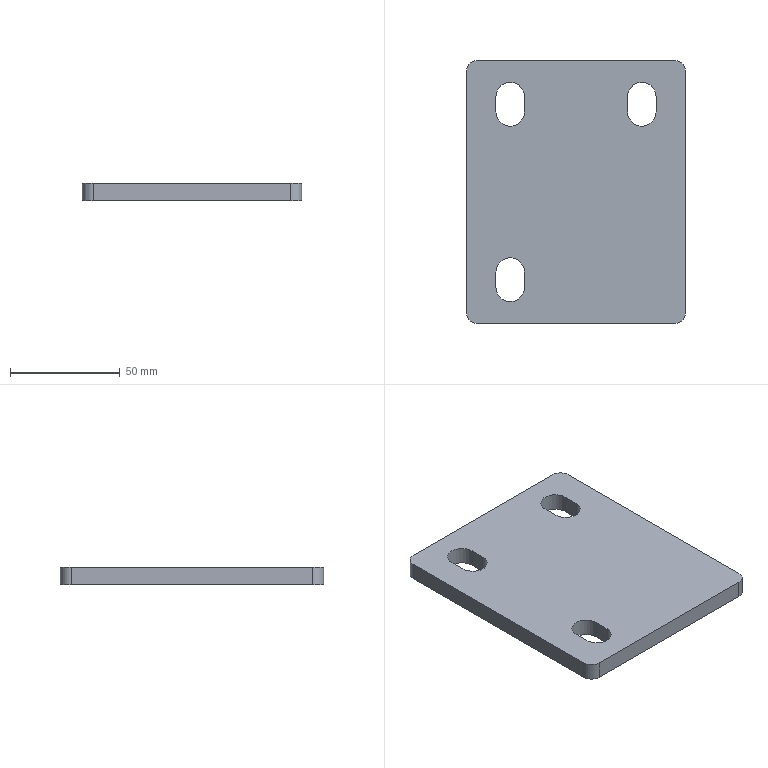Part | STEP file | HL4GD-1.30.106 cab frame side mounting plate-
-20251212 | 1 solid | 22 faces | box 100 x 120 x 8 mm | volume 90459 mm3 | plane 12 | cylinder 10 | commonest cylinder face diameters 13 x6 10 x4